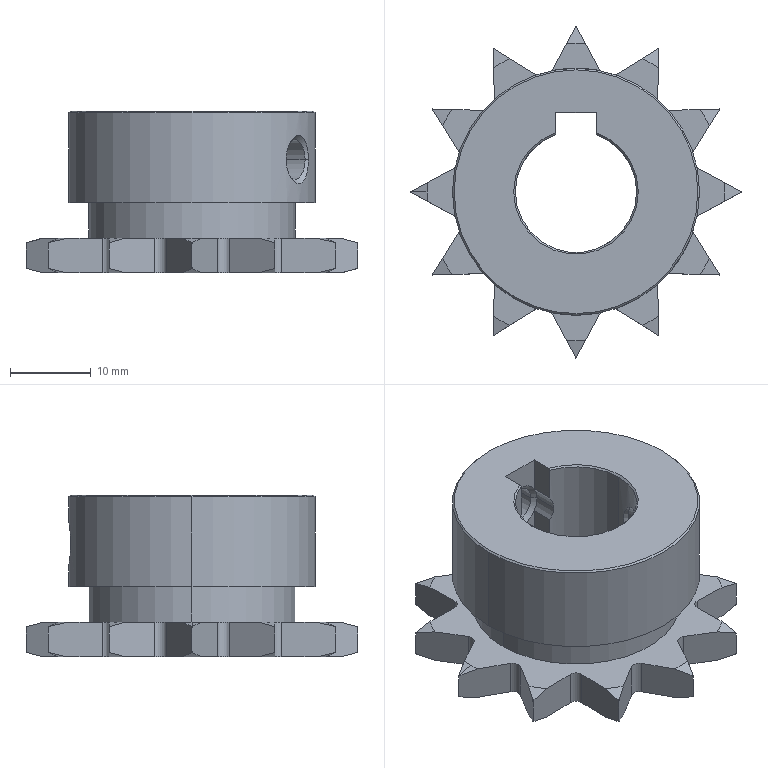Part | STEP file | SP35B12_N_15_SP35B12-N-15 | 1 solid | 135 faces | box 41 x 41 x 20 mm | volume 10343 mm3 | cone 42 | plane 34 | cylinder 33 | torus 26 | commonest cylinder face diameters 2 x16 6 x6 4.917 x4 15 x3 25.5 x2 30.5 x2